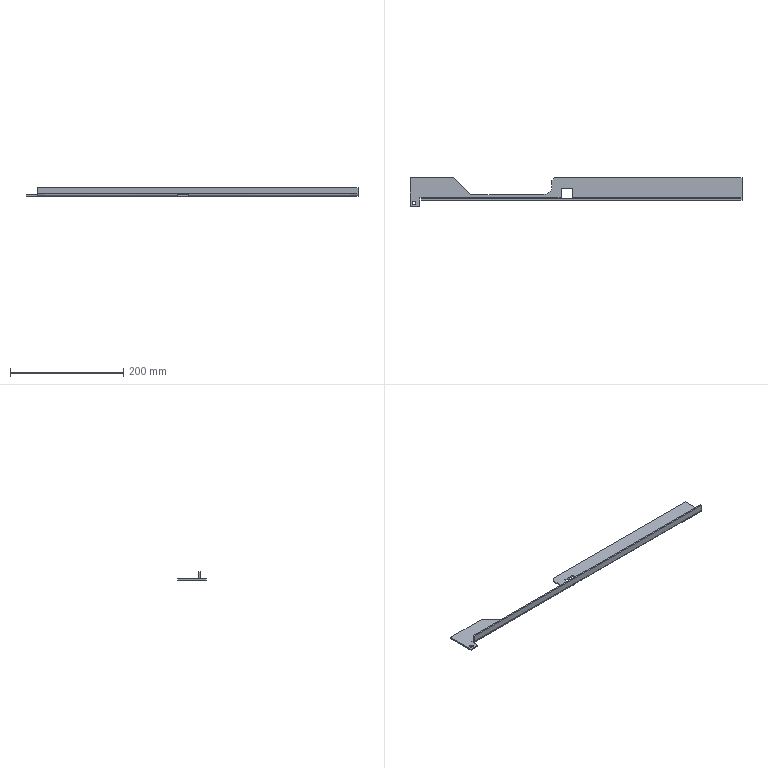Part | STEP file | 1 solid | 27 faces | box 587 x 51 x 15 mm | volume 62244 mm3 | plane 21 | cylinder 6 | commonest cylinder face diameters 6 x2 3 x1 8 x1 20 x1 30 x1